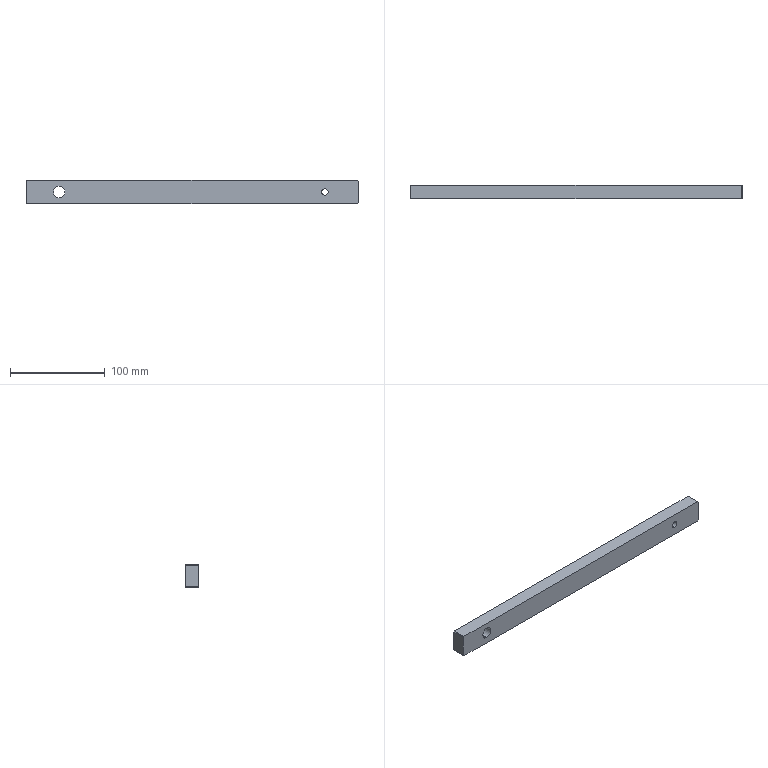Part | SolidWorks | features FlatPattern 1, HoleWzd 1, SMBaseFlange 1, SheetMetal 1 | 1 solid | 14 faces | box 350 x 14 x 25 mm | volume 120380 mm3 | plane 10 | cylinder 4 | commonest cylinder face diameters 6.8 x2 12 x2
STEP:
#1=CARTESIAN_POINT('',(140.,0.,3.4));
#2=VERTEX_POINT('',#1);
#3=CARTESIAN_POINT('',(140.,0.,-3.4));
#4=VERTEX_POINT('',#3);
#5=CARTESIAN_POINT('',(140.,0.,0.));
#6=DIRECTION('',(0.,-1.,0.));
#7=DIRECTION('',(0.,0.,-1.));
#8=AXIS2_PLACEMENT_3D('',#5,#6,#7);
#9=CIRCLE('',#8,3.4);
#10=EDGE_CURVE('',#2,#4,#9,.T.);
#11=ORIENTED_EDGE('',*,*,#10,.T.);
#12=CARTESIAN_POINT('',(140.,14.,-3.4));
#13=VERTEX_POINT('',#12);
#14=CARTESIAN_POINT('',(140.,14.,-3.4));
#15=DIRECTION('',(0.,1.,0.));
#16=VECTOR('',#15,1000.);
#17=LINE('',#14,#16);
#18=EDGE_CURVE('',#4,#13,#17,.T.);
#19=ORIENTED_EDGE('',*,*,#18,.T.);
#20=CARTESIAN_POINT('',(140.,14.,3.4));
#21=VERTEX_POINT('',#20);
#22=CARTESIAN_POINT('',(140.,14.,0.));
#23=DIRECTION('',(0.,1.,0.));
#24=DIRECTION('',(0.,0.,1.));
#25=AXIS2_PLACEMENT_3D('',#22,#23,#24);
#26=CIRCLE('',#25,3.4);
#27=EDGE_CURVE('',#13,#21,#26,.T.);
#28=ORIENTED_EDGE('',*,*,#27,.T.);
#29=CARTESIAN_POINT('',(140.,14.,3.4));
#30=DIRECTION('',(0.,1.,0.));
#31=VECTOR('',#30,1000.);
#32=LINE('',#29,#31);
#33=EDGE_CURVE('',#2,#21,#32,.T.);
#34=ORIENTED_EDGE('',*,*,#33,.F.);
#35=EDGE_LOOP('',(#11,#19,#28,#34));
#36=FACE_OUTER_BOUND('',#35,.T.);
#37=CARTESIAN_POINT('',(140.,14.,0.));
#38=DIRECTION('',(0.,1.,0.));
#39=DIRECTION('',(0.,0.,1.));
#40=AXIS2_PLACEMENT_3D('',#37,#38,#39);
#41=CYLINDRICAL_SURFACE('',#40,3.4);
#42=ADVANCED_FACE('',(#36),#41,.F.);
#43=CARTESIAN_POINT('',(-140.,14.,-6.));
#44=VERTEX_POINT('',#43);
#45=CARTESIAN_POINT('',(-140.,14.,6.));
#46=VERTEX_POINT('',#45);
#47=CARTESIAN_POINT('',(-140.,14.,0.));
#48=DIRECTION('',(0.,1.,0.));
#49=DIRECTION('',(0.,0.,1.));
#50=AXIS2_PLACEMENT_3D('',#47,#48,#49);
#51=CIRCLE('',#50,6.);
#52=EDGE_CURVE('',#44,#46,#51,.T.);
#53=ORIENTED_EDGE('',*,*,#52,.T.);
#54=CARTESIAN_POINT('',(-140.,0.,6.));
#55=VERTEX_POINT('',#54);
#56=CARTESIAN_POINT('',(-140.,14.,6.));
#57=DIRECTION('',(0.,-1.,0.));
#58=VECTOR('',#57,1000.);
#59=LINE('',#56,#58);
#60=EDGE_CURVE('',#46,#55,#59,.T.);
#61=ORIENTED_EDGE('',*,*,#60,.T.);
#62=CARTESIAN_POINT('',(-140.,0.,-6.));
#63=VERTEX_POINT('',#62);
#64=CARTESIAN_POINT('',(-140.,0.,0.));
#65=DIRECTION('',(0.,1.,0.));
#66=DIRECTION('',(0.,0.,1.));
#67=AXIS2_PLACEMENT_3D('',#64,#65,#66);
#68=CIRCLE('',#67,6.);
#69=EDGE_CURVE('',#63,#55,#68,.T.);
#70=ORIENTED_EDGE('',*,*,#69,.F.);
#71=CARTESIAN_POINT('',(-140.,14.,-6.));
#72=DIRECTION('',(0.,-1.,0.));
#73=VECTOR('',#72,1000.);
#74=LINE('',#71,#73);
#75=EDGE_CURVE('',#44,#63,#74,.T.);
#76=ORIENTED_EDGE('',*,*,#75,.F.);
#77=EDGE_LOOP('',(#53,#61,#70,#76));
#78=FACE_OUTER_BOUND('',#77,.T.);
#79=CARTESIAN_POINT('',(-140.,14.,0.));
#80=DIRECTION('',(0.,-1.,0.));
#81=DIRECTION('',(0.,0.,-1.));
#82=AXIS2_PLACEMENT_3D('',#79,#80,#81);
#83=CYLINDRICAL_SURFACE('',#82,6.);
#84=ADVANCED_FACE('',(#78),#83,.F.);
#85=CARTESIAN_POINT('',(140.,14.,0.));
#86=DIRECTION('',(0.,1.,0.));
#87=DIRECTION('',(0.,0.,1.));
#88=AXIS2_PLACEMENT_3D('',#85,#86,#87);
#89=CIRCLE('',#88,3.4);
#90=EDGE_CURVE('',#21,#13,#89,.T.);
#91=ORIENTED_EDGE('',*,*,#90,.F.);
#92=ORIENTED_EDGE('',*,*,#27,.F.);
#93=EDGE_LOOP('',(#91,#92));
#94=FACE_BOUND('',#93,.T.);
#95=CARTESIAN_POINT('',(174.,14.,-12.5));
#96=VERTEX_POINT('',#95);
#97=CARTESIAN_POINT('',(-174.,14.,-12.5));
#98=VERTEX_POINT('',#97);
#99=CARTESIAN_POINT('',(-174.,14.,-12.5));
#100=DIRECTION('',(-1.,0.,0.));
#101=VECTOR('',#100,1000.);
#102=LINE('',#99,#101);
#103=EDGE_CURVE('',#96,#98,#102,.T.);
#104=ORIENTED_EDGE('',*,*,#103,.T.);
#105=CARTESIAN_POINT('',(-175.,14.,-11.5));
#106=VERTEX_POINT('',#105);
#107=CARTESIAN_POINT('',(-175.,14.,-11.5));
#108=DIRECTION('',(-0.7071,0.,0.7071));
#109=VECTOR('',#108,1000.);
#110=LINE('',#107,#109);
#111=EDGE_CURVE('',#98,#106,#110,.T.);
#112=ORIENTED_EDGE('',*,*,#111,.T.);
#113=CARTESIAN_POINT('',(-175.,14.,11.5));
#114=VERTEX_POINT('',#113);
#115=CARTESIAN_POINT('',(-175.,14.,-11.5));
#116=DIRECTION('',(0.,0.,1.));
#117=VECTOR('',#116,1000.);
#118=LINE('',#115,#117);
#119=EDGE_CURVE('',#106,#114,#118,.T.);
#120=ORIENTED_EDGE('',*,*,#119,.T.);
#121=CARTESIAN_POINT('',(-174.,14.,12.5));
#122=VERTEX_POINT('',#121);
#123=CARTESIAN_POINT('',(-175.,14.,11.5));
#124=DIRECTION('',(0.7071,0.,0.7071));
#125=VECTOR('',#124,1000.);
#126=LINE('',#123,#125);
#127=EDGE_CURVE('',#114,#122,#126,.T.);
#128=ORIENTED_EDGE('',*,*,#127,.T.);
#129=CARTESIAN_POINT('',(174.,14.,12.5));
#130=VERTEX_POINT('',#129);
#131=CARTESIAN_POINT('',(-174.,14.,12.5));
#132=DIRECTION('',(1.,0.,0.));
#133=VECTOR('',#132,1000.);
#134=LINE('',#131,#133);
#135=EDGE_CURVE('',#122,#130,#134,.T.);
#136=ORIENTED_EDGE('',*,*,#135,.T.);
#137=CARTESIAN_POINT('',(175.,14.,11.5));
#138=VERTEX_POINT('',#137);
#139=CARTESIAN_POINT('',(174.,14.,12.5));
#140=DIRECTION('',(0.7071,0.,-0.7071));
#141=VECTOR('',#140,1000.);
#142=LINE('',#139,#141);
#143=EDGE_CURVE('',#130,#138,#142,.T.);
#144=ORIENTED_EDGE('',*,*,#143,.T.);
#145=CARTESIAN_POINT('',(175.,14.,-11.5));
#146=VERTEX_POINT('',#145);
#147=CARTESIAN_POINT('',(175.,14.,-11.5));
#148=DIRECTION('',(0.,0.,-1.));
#149=VECTOR('',#148,1000.);
#150=LINE('',#147,#149);
#151=EDGE_CURVE('',#138,#146,#150,.T.);
#152=ORIENTED_EDGE('',*,*,#151,.T.);
#153=CARTESIAN_POINT('',(174.,14.,-12.5));
#154=DIRECTION('',(-0.7071,0.,-0.7071));
#155=VECTOR('',#154,1000.);
#156=LINE('',#153,#155);
#157=EDGE_CURVE('',#146,#96,#156,.T.);
#158=ORIENTED_EDGE('',*,*,#157,.T.);
#159=EDGE_LOOP('',(#104,#112,#120,#128,#136,#144,#152,#158));
#160=FACE_OUTER_BOUND('',#159,.T.);
#161=ORIENTED_EDGE('',*,*,#52,.F.);
#162=CARTESIAN_POINT('',(-140.,14.,0.));
#163=DIRECTION('',(0.,1.,0.));
#164=DIRECTION('',(0.,0.,1.));
#165=AXIS2_PLACEMENT_3D('',#162,#163,#164);
#166=CIRCLE('',#165,6.);
#167=EDGE_CURVE('',#46,#44,#166,.T.);
#168=ORIENTED_EDGE('',*,*,#167,.F.);
#169=EDGE_LOOP('',(#161,#168));
#170=FACE_BOUND('',#169,.T.);
#171=CARTESIAN_POINT('',(0.,14.,0.));
#172=DIRECTION('',(0.,-1.,0.));
#173=DIRECTION('',(0.,0.,-1.));
#174=AXIS2_PLACEMENT_3D('',#171,#172,#173);
#175=PLANE('',#174);
#176=ADVANCED_FACE('',(#94,#160,#170),#175,.F.);
#177=ORIENTED_EDGE('',*,*,#10,.F.);
#178=CARTESIAN_POINT('',(140.,0.,0.));
#179=DIRECTION('',(0.,-1.,0.));
#180=DIRECTION('',(0.,0.,-1.));
#181=AXIS2_PLACEMENT_3D('',#178,#179,#180);
#182=CIRCLE('',#181,3.4);
#183=EDGE_CURVE('',#4,#2,#182,.T.);
#184=ORIENTED_EDGE('',*,*,#183,.F.);
#185=EDGE_LOOP('',(#177,#184));
#186=FACE_BOUND('',#185,.T.);
#187=ORIENTED_EDGE('',*,*,#69,.T.);
#188=CARTESIAN_POINT('',(-140.,0.,0.));
#189=DIRECTION('',(0.,1.,0.));
#190=DIRECTION('',(0.,0.,1.));
#191=AXIS2_PLACEMENT_3D('',#188,#189,#190);
#192=CIRCLE('',#191,6.);
#193=EDGE_CURVE('',#55,#63,#192,.T.);
#194=ORIENTED_EDGE('',*,*,#193,.T.);
#195=EDGE_LOOP('',(#187,#194));
#196=FACE_BOUND('',#195,.T.);
#197=CARTESIAN_POINT('',(174.,0.,-12.5));
#198=VERTEX_POINT('',#197);
#199=CARTESIAN_POINT('',(-174.,0.,-12.5));
#200=VERTEX_POINT('',#199);
#201=CARTESIAN_POINT('',(-174.,0.,-12.5));
#202=DIRECTION('',(-1.,0.,0.));
#203=VECTOR('',#202,1000.);
#204=LINE('',#201,#203);
#205=EDGE_CURVE('',#198,#200,#204,.T.);
#206=ORIENTED_EDGE('',*,*,#205,.F.);
#207=CARTESIAN_POINT('',(175.,0.,-11.5));
#208=VERTEX_POINT('',#207);
#209=CARTESIAN_POINT('',(174.,0.,-12.5));
#210=DIRECTION('',(-0.7071,0.,-0.7071));
#211=VECTOR('',#210,1000.);
#212=LINE('',#209,#211);
#213=EDGE_CURVE('',#208,#198,#212,.T.);
#214=ORIENTED_EDGE('',*,*,#213,.F.);
#215=CARTESIAN_POINT('',(175.,0.,11.5));
#216=VERTEX_POINT('',#215);
#217=CARTESIAN_POINT('',(175.,0.,-11.5));
#218=DIRECTION('',(0.,0.,-1.));
#219=VECTOR('',#218,1000.);
#220=LINE('',#217,#219);
#221=EDGE_CURVE('',#216,#208,#220,.T.);
#222=ORIENTED_EDGE('',*,*,#221,.F.);
#223=CARTESIAN_POINT('',(174.,0.,12.5));
#224=VERTEX_POINT('',#223);
#225=CARTESIAN_POINT('',(174.,0.,12.5));
#226=DIRECTION('',(0.7071,0.,-0.7071));
#227=VECTOR('',#226,1000.);
#228=LINE('',#225,#227);
#229=EDGE_CURVE('',#224,#216,#228,.T.);
#230=ORIENTED_EDGE('',*,*,#229,.F.);
#231=CARTESIAN_POINT('',(-174.,0.,12.5));
#232=VERTEX_POINT('',#231);
#233=CARTESIAN_POINT('',(-174.,0.,12.5));
#234=DIRECTION('',(1.,0.,0.));
#235=VECTOR('',#234,1000.);
#236=LINE('',#233,#235);
#237=EDGE_CURVE('',#232,#224,#236,.T.);
#238=ORIENTED_EDGE('',*,*,#237,.F.);
#239=CARTESIAN_POINT('',(-175.,0.,11.5));
#240=VERTEX_POINT('',#239);
#241=CARTESIAN_POINT('',(-175.,0.,11.5));
#242=DIRECTION('',(0.7071,0.,0.7071));
#243=VECTOR('',#242,1000.);
#244=LINE('',#241,#243);
#245=EDGE_CURVE('',#240,#232,#244,.T.);
#246=ORIENTED_EDGE('',*,*,#245,.F.);
#247=CARTESIAN_POINT('',(-175.,0.,-11.5));
#248=VERTEX_POINT('',#247);
#249=CARTESIAN_POINT('',(-175.,0.,-11.5));
#250=DIRECTION('',(0.,0.,1.));
#251=VECTOR('',#250,1000.);
#252=LINE('',#249,#251);
#253=EDGE_CURVE('',#248,#240,#252,.T.);
#254=ORIENTED_EDGE('',*,*,#253,.F.);
#255=CARTESIAN_POINT('',(-175.,0.,-11.5));
#256=DIRECTION('',(-0.7071,0.,0.7071));
#257=VECTOR('',#256,1000.);
#258=LINE('',#255,#257);
#259=EDGE_CURVE('',#200,#248,#258,.T.);
#260=ORIENTED_EDGE('',*,*,#259,.F.);
#261=EDGE_LOOP('',(#206,#214,#222,#230,#238,#246,#254,#260));
#262=FACE_OUTER_BOUND('',#261,.T.);
#263=CARTESIAN_POINT('',(0.,0.,0.));
#264=DIRECTION('',(0.,-1.,0.));
#265=DIRECTION('',(0.,0.,-1.));
#266=AXIS2_PLACEMENT_3D('',#263,#264,#265);
#267=PLANE('',#266);
#268=ADVANCED_FACE('',(#186,#196,#262),#267,.T.);
#269=ORIENTED_EDGE('',*,*,#205,.T.);
#270=CARTESIAN_POINT('',(-174.,14.,-12.5));
#271=DIRECTION('',(0.,-1.,0.));
#272=VECTOR('',#271,1000.);
#273=LINE('',#270,#272);
#274=EDGE_CURVE('',#98,#200,#273,.T.);
#275=ORIENTED_EDGE('',*,*,#274,.F.);
#276=ORIENTED_EDGE('',*,*,#103,.F.);
#277=CARTESIAN_POINT('',(174.,14.,-12.5));
#278=DIRECTION('',(0.,-1.,0.));
#279=VECTOR('',#278,1000.);
#280=LINE('',#277,#279);
#281=EDGE_CURVE('',#96,#198,#280,.T.);
#282=ORIENTED_EDGE('',*,*,#281,.T.);
#283=EDGE_LOOP('',(#269,#275,#276,#282));
#284=FACE_OUTER_BOUND('',#283,.T.);
#285=CARTESIAN_POINT('',(-174.,14.,-12.5));
#286=DIRECTION('',(0.,0.,1.));
#287=DIRECTION('',(1.,0.,0.));
#288=AXIS2_PLACEMENT_3D('',#285,#286,#287);
#289=PLANE('',#288);
#290=ADVANCED_FACE('',(#284),#289,.F.);
#291=ORIENTED_EDGE('',*,*,#259,.T.);
#292=CARTESIAN_POINT('',(-175.,14.,-11.5));
#293=DIRECTION('',(0.,-1.,0.));
#294=VECTOR('',#293,1000.);
#295=LINE('',#292,#294);
#296=EDGE_CURVE('',#106,#248,#295,.T.);
#297=ORIENTED_EDGE('',*,*,#296,.F.);
#298=ORIENTED_EDGE('',*,*,#111,.F.);
#299=ORIENTED_EDGE('',*,*,#274,.T.);
#300=EDGE_LOOP('',(#291,#297,#298,#299));
#301=FACE_OUTER_BOUND('',#300,.T.);
#302=CARTESIAN_POINT('',(-175.,14.,-11.5));
#303=DIRECTION('',(0.7071,0.,0.7071));
#304=DIRECTION('',(0.7071,0.,-0.7071));
#305=AXIS2_PLACEMENT_3D('',#302,#303,#304);
#306=PLANE('',#305);
#307=ADVANCED_FACE('',(#301),#306,.F.);
#308=ORIENTED_EDGE('',*,*,#253,.T.);
#309=CARTESIAN_POINT('',(-175.,14.,11.5));
#310=DIRECTION('',(0.,-1.,0.));
#311=VECTOR('',#310,1000.);
#312=LINE('',#309,#311);
#313=EDGE_CURVE('',#114,#240,#312,.T.);
#314=ORIENTED_EDGE('',*,*,#313,.F.);
#315=ORIENTED_EDGE('',*,*,#119,.F.);
#316=ORIENTED_EDGE('',*,*,#296,.T.);
#317=EDGE_LOOP('',(#308,#314,#315,#316));
#318=FACE_OUTER_BOUND('',#317,.T.);
#319=CARTESIAN_POINT('',(-175.,14.,-11.5));
#320=DIRECTION('',(1.,0.,0.));
#321=DIRECTION('',(0.,0.,-1.));
#322=AXIS2_PLACEMENT_3D('',#319,#320,#321);
#323=PLANE('',#322);
#324=ADVANCED_FACE('',(#318),#323,.F.);
#325=ORIENTED_EDGE('',*,*,#245,.T.);
#326=CARTESIAN_POINT('',(-174.,14.,12.5));
#327=DIRECTION('',(0.,-1.,0.));
#328=VECTOR('',#327,1000.);
#329=LINE('',#326,#328);
#330=EDGE_CURVE('',#122,#232,#329,.T.);
#331=ORIENTED_EDGE('',*,*,#330,.F.);
#332=ORIENTED_EDGE('',*,*,#127,.F.);
#333=ORIENTED_EDGE('',*,*,#313,.T.);
#334=EDGE_LOOP('',(#325,#331,#332,#333));
#335=FACE_OUTER_BOUND('',#334,.T.);
#336=CARTESIAN_POINT('',(-175.,14.,11.5));
#337=DIRECTION('',(0.7071,0.,-0.7071));
#338=DIRECTION('',(-0.7071,0.,-0.7071));
#339=AXIS2_PLACEMENT_3D('',#336,#337,#338);
#340=PLANE('',#339);
#341=ADVANCED_FACE('',(#335),#340,.F.);
#342=ORIENTED_EDGE('',*,*,#237,.T.);
#343=CARTESIAN_POINT('',(174.,14.,12.5));
#344=DIRECTION('',(0.,-1.,0.));
#345=VECTOR('',#344,1000.);
#346=LINE('',#343,#345);
#347=EDGE_CURVE('',#130,#224,#346,.T.);
#348=ORIENTED_EDGE('',*,*,#347,.F.);
#349=ORIENTED_EDGE('',*,*,#135,.F.);
#350=ORIENTED_EDGE('',*,*,#330,.T.);
#351=EDGE_LOOP('',(#342,#348,#349,#350));
#352=FACE_OUTER_BOUND('',#351,.T.);
#353=CARTESIAN_POINT('',(-174.,14.,12.5));
#354=DIRECTION('',(0.,0.,-1.));
#355=DIRECTION('',(-1.,0.,0.));
#356=AXIS2_PLACEMENT_3D('',#353,#354,#355);
#357=PLANE('',#356);
#358=ADVANCED_FACE('',(#352),#357,.F.);
#359=ORIENTED_EDGE('',*,*,#229,.T.);
#360=CARTESIAN_POINT('',(175.,14.,11.5));
#361=DIRECTION('',(0.,-1.,0.));
#362=VECTOR('',#361,1000.);
#363=LINE('',#360,#362);
#364=EDGE_CURVE('',#138,#216,#363,.T.);
#365=ORIENTED_EDGE('',*,*,#364,.F.);
#366=ORIENTED_EDGE('',*,*,#143,.F.);
#367=ORIENTED_EDGE('',*,*,#347,.T.);
#368=EDGE_LOOP('',(#359,#365,#366,#367));
#369=FACE_OUTER_BOUND('',#368,.T.);
#370=CARTESIAN_POINT('',(174.,14.,12.5));
#371=DIRECTION('',(-0.7071,0.,-0.7071));
#372=DIRECTION('',(-0.7071,0.,0.7071));
#373=AXIS2_PLACEMENT_3D('',#370,#371,#372);
#374=PLANE('',#373);
#375=ADVANCED_FACE('',(#369),#374,.F.);
#376=ORIENTED_EDGE('',*,*,#221,.T.);
#377=CARTESIAN_POINT('',(175.,14.,-11.5));
#378=DIRECTION('',(0.,-1.,0.));
#379=VECTOR('',#378,1000.);
#380=LINE('',#377,#379);
#381=EDGE_CURVE('',#146,#208,#380,.T.);
#382=ORIENTED_EDGE('',*,*,#381,.F.);
#383=ORIENTED_EDGE('',*,*,#151,.F.);
#384=ORIENTED_EDGE('',*,*,#364,.T.);
#385=EDGE_LOOP('',(#376,#382,#383,#384));
#386=FACE_OUTER_BOUND('',#385,.T.);
#387=CARTESIAN_POINT('',(175.,14.,-11.5));
#388=DIRECTION('',(-1.,0.,0.));
#389=DIRECTION('',(0.,0.,1.));
#390=AXIS2_PLACEMENT_3D('',#387,#388,#389);
#391=PLANE('',#390);
#392=ADVANCED_FACE('',(#386),#391,.F.);
#393=ORIENTED_EDGE('',*,*,#213,.T.);
#394=ORIENTED_EDGE('',*,*,#281,.F.);
#395=ORIENTED_EDGE('',*,*,#157,.F.);
#396=ORIENTED_EDGE('',*,*,#381,.T.);
#397=EDGE_LOOP('',(#393,#394,#395,#396));
#398=FACE_OUTER_BOUND('',#397,.T.);
#399=CARTESIAN_POINT('',(174.,14.,-12.5));
#400=DIRECTION('',(-0.7071,0.,0.7071));
#401=DIRECTION('',(0.7071,0.,0.7071));
#402=AXIS2_PLACEMENT_3D('',#399,#400,#401);
#403=PLANE('',#402);
#404=ADVANCED_FACE('',(#398),#403,.F.);
#405=ORIENTED_EDGE('',*,*,#60,.F.);
#406=ORIENTED_EDGE('',*,*,#167,.T.);
#407=ORIENTED_EDGE('',*,*,#75,.T.);
#408=ORIENTED_EDGE('',*,*,#193,.F.);
#409=EDGE_LOOP('',(#405,#406,#407,#408));
#410=FACE_OUTER_BOUND('',#409,.T.);
#411=CARTESIAN_POINT('',(-140.,14.,0.));
#412=DIRECTION('',(0.,-1.,0.));
#413=DIRECTION('',(0.,0.,-1.));
#414=AXIS2_PLACEMENT_3D('',#411,#412,#413);
#415=CYLINDRICAL_SURFACE('',#414,6.);
#416=ADVANCED_FACE('',(#410),#415,.F.);
#417=ORIENTED_EDGE('',*,*,#18,.F.);
#418=ORIENTED_EDGE('',*,*,#183,.T.);
#419=ORIENTED_EDGE('',*,*,#33,.T.);
#420=ORIENTED_EDGE('',*,*,#90,.T.);
#421=EDGE_LOOP('',(#417,#418,#419,#420));
#422=FACE_OUTER_BOUND('',#421,.T.);
#423=CARTESIAN_POINT('',(140.,14.,0.));
#424=DIRECTION('',(0.,1.,0.));
#425=DIRECTION('',(0.,0.,1.));
#426=AXIS2_PLACEMENT_3D('',#423,#424,#425);
#427=CYLINDRICAL_SURFACE('',#426,3.4);
#428=ADVANCED_FACE('',(#422),#427,.F.);
#429=CLOSED_SHELL('',(#42,#84,#176,#268,#290,#307,#324,#341,#358,#375,#392,#404,#416,#428));
#430=MANIFOLD_SOLID_BREP('',#429);
#431=CARTESIAN_POINT('',(0.,0.,0.));
#432=DIRECTION('',(0.,0.,1.));
#433=DIRECTION('',(1.,0.,0.));
#434=AXIS2_PLACEMENT_3D('',#431,#432,#433);
#435=(LENGTH_UNIT()NAMED_UNIT(*)SI_UNIT(.MILLI.,.METRE.));
#436=UNCERTAINTY_MEASURE_WITH_UNIT(LENGTH_MEASURE(0.00001),#435,'','');
#437=(NAMED_UNIT(*)PLANE_ANGLE_UNIT()SI_UNIT($,.RADIAN.));
#438=(NAMED_UNIT(*)SI_UNIT($,.STERADIAN.)SOLID_ANGLE_UNIT());
#439=(GEOMETRIC_REPRESENTATION_CONTEXT(3)GLOBAL_UNCERTAINTY_ASSIGNED_CONTEXT((#436))GLOBAL_UNIT_ASSIGNED_CONTEXT((#435,#437,#438))REPRESENTATION_CONTEXT('',''));
#440=ADVANCED_BREP_SHAPE_REPRESENTATION('',(#430,#434),#439);